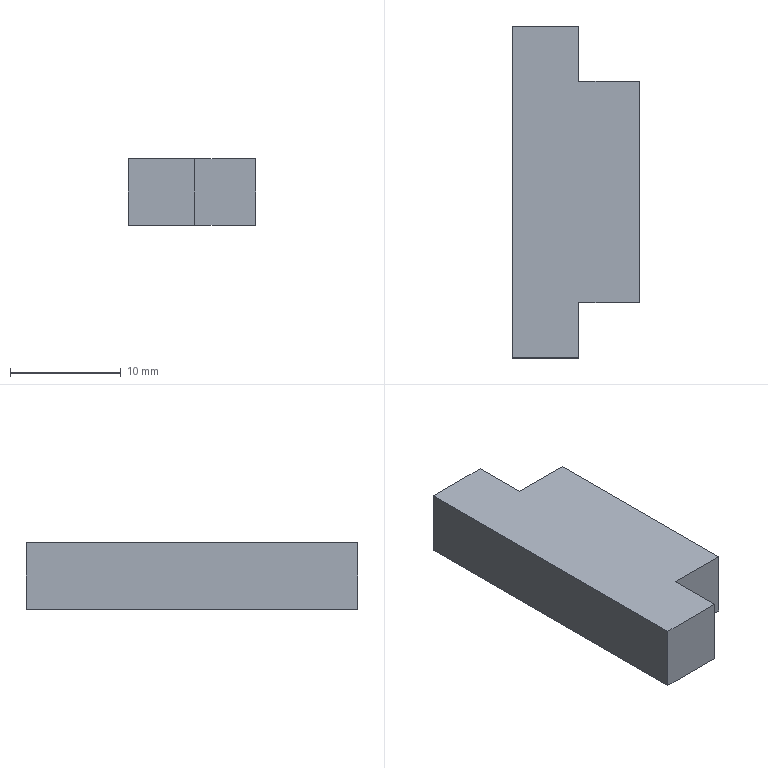Part | SolidWorks | features FlatPattern 1, SMBaseFlange 1, SheetMetal 1 | 1 solid | 10 faces | box 11.5 x 30 x 6 mm | volume 1740 mm3 | plane 10
STEP:
#1=CARTESIAN_POINT('',(11.5,-104.,0.));
#2=VERTEX_POINT('',#1);
#3=CARTESIAN_POINT('',(11.5,-84.,0.));
#4=VERTEX_POINT('',#3);
#5=CARTESIAN_POINT('',(11.5,-84.,0.));
#6=DIRECTION('',(0.,1.,0.));
#7=VECTOR('',#6,1000.);
#8=LINE('',#5,#7);
#9=EDGE_CURVE('',#2,#4,#8,.T.);
#10=ORIENTED_EDGE('',*,*,#9,.T.);
#11=CARTESIAN_POINT('',(11.5,-84.,6.));
#12=VERTEX_POINT('',#11);
#13=CARTESIAN_POINT('',(11.5,-84.,6.));
#14=DIRECTION('',(0.,0.,-1.));
#15=VECTOR('',#14,1000.);
#16=LINE('',#13,#15);
#17=EDGE_CURVE('',#12,#4,#16,.T.);
#18=ORIENTED_EDGE('',*,*,#17,.F.);
#19=CARTESIAN_POINT('',(11.5,-104.,6.));
#20=VERTEX_POINT('',#19);
#21=CARTESIAN_POINT('',(11.5,-84.,6.));
#22=DIRECTION('',(0.,1.,0.));
#23=VECTOR('',#22,1000.);
#24=LINE('',#21,#23);
#25=EDGE_CURVE('',#20,#12,#24,.T.);
#26=ORIENTED_EDGE('',*,*,#25,.F.);
#27=CARTESIAN_POINT('',(11.5,-104.,6.));
#28=DIRECTION('',(0.,0.,-1.));
#29=VECTOR('',#28,1000.);
#30=LINE('',#27,#29);
#31=EDGE_CURVE('',#20,#2,#30,.T.);
#32=ORIENTED_EDGE('',*,*,#31,.T.);
#33=EDGE_LOOP('',(#10,#18,#26,#32));
#34=FACE_OUTER_BOUND('',#33,.T.);
#35=CARTESIAN_POINT('',(11.5,-84.,6.));
#36=DIRECTION('',(-1.,0.,0.));
#37=DIRECTION('',(0.,-1.,0.));
#38=AXIS2_PLACEMENT_3D('',#35,#36,#37);
#39=PLANE('',#38);
#40=ADVANCED_FACE('',(#34),#39,.F.);
#41=CARTESIAN_POINT('',(6.,-84.,0.));
#42=VERTEX_POINT('',#41);
#43=CARTESIAN_POINT('',(6.,-84.,0.));
#44=DIRECTION('',(-1.,0.,0.));
#45=VECTOR('',#44,1000.);
#46=LINE('',#43,#45);
#47=EDGE_CURVE('',#4,#42,#46,.T.);
#48=ORIENTED_EDGE('',*,*,#47,.T.);
#49=CARTESIAN_POINT('',(6.,-84.,6.));
#50=VERTEX_POINT('',#49);
#51=CARTESIAN_POINT('',(6.,-84.,6.));
#52=DIRECTION('',(0.,0.,-1.));
#53=VECTOR('',#52,1000.);
#54=LINE('',#51,#53);
#55=EDGE_CURVE('',#50,#42,#54,.T.);
#56=ORIENTED_EDGE('',*,*,#55,.F.);
#57=CARTESIAN_POINT('',(6.,-84.,6.));
#58=DIRECTION('',(-1.,0.,0.));
#59=VECTOR('',#58,1000.);
#60=LINE('',#57,#59);
#61=EDGE_CURVE('',#12,#50,#60,.T.);
#62=ORIENTED_EDGE('',*,*,#61,.F.);
#63=ORIENTED_EDGE('',*,*,#17,.T.);
#64=EDGE_LOOP('',(#48,#56,#62,#63));
#65=FACE_OUTER_BOUND('',#64,.T.);
#66=CARTESIAN_POINT('',(6.,-84.,6.));
#67=DIRECTION('',(0.,-1.,0.));
#68=DIRECTION('',(0.,0.,-1.));
#69=AXIS2_PLACEMENT_3D('',#66,#67,#68);
#70=PLANE('',#69);
#71=ADVANCED_FACE('',(#65),#70,.F.);
#72=CARTESIAN_POINT('',(6.,-79.,0.));
#73=VERTEX_POINT('',#72);
#74=CARTESIAN_POINT('',(6.,-79.,0.));
#75=DIRECTION('',(0.,1.,0.));
#76=VECTOR('',#75,1000.);
#77=LINE('',#74,#76);
#78=EDGE_CURVE('',#42,#73,#77,.T.);
#79=ORIENTED_EDGE('',*,*,#78,.T.);
#80=CARTESIAN_POINT('',(6.,-79.,6.));
#81=VERTEX_POINT('',#80);
#82=CARTESIAN_POINT('',(6.,-79.,6.));
#83=DIRECTION('',(0.,0.,-1.));
#84=VECTOR('',#83,1000.);
#85=LINE('',#82,#84);
#86=EDGE_CURVE('',#81,#73,#85,.T.);
#87=ORIENTED_EDGE('',*,*,#86,.F.);
#88=CARTESIAN_POINT('',(6.,-79.,6.));
#89=DIRECTION('',(0.,1.,0.));
#90=VECTOR('',#89,1000.);
#91=LINE('',#88,#90);
#92=EDGE_CURVE('',#50,#81,#91,.T.);
#93=ORIENTED_EDGE('',*,*,#92,.F.);
#94=ORIENTED_EDGE('',*,*,#55,.T.);
#95=EDGE_LOOP('',(#79,#87,#93,#94));
#96=FACE_OUTER_BOUND('',#95,.T.);
#97=CARTESIAN_POINT('',(6.,-79.,6.));
#98=DIRECTION('',(-1.,0.,0.));
#99=DIRECTION('',(0.,-1.,0.));
#100=AXIS2_PLACEMENT_3D('',#97,#98,#99);
#101=PLANE('',#100);
#102=ADVANCED_FACE('',(#96),#101,.F.);
#103=CARTESIAN_POINT('',(0.,-79.,0.));
#104=VERTEX_POINT('',#103);
#105=CARTESIAN_POINT('',(0.,-79.,0.));
#106=DIRECTION('',(-1.,0.,0.));
#107=VECTOR('',#106,1000.);
#108=LINE('',#105,#107);
#109=EDGE_CURVE('',#73,#104,#108,.T.);
#110=ORIENTED_EDGE('',*,*,#109,.T.);
#111=CARTESIAN_POINT('',(0.,-79.,6.));
#112=VERTEX_POINT('',#111);
#113=CARTESIAN_POINT('',(0.,-79.,6.));
#114=DIRECTION('',(0.,0.,-1.));
#115=VECTOR('',#114,1000.);
#116=LINE('',#113,#115);
#117=EDGE_CURVE('',#112,#104,#116,.T.);
#118=ORIENTED_EDGE('',*,*,#117,.F.);
#119=CARTESIAN_POINT('',(0.,-79.,6.));
#120=DIRECTION('',(-1.,0.,0.));
#121=VECTOR('',#120,1000.);
#122=LINE('',#119,#121);
#123=EDGE_CURVE('',#81,#112,#122,.T.);
#124=ORIENTED_EDGE('',*,*,#123,.F.);
#125=ORIENTED_EDGE('',*,*,#86,.T.);
#126=EDGE_LOOP('',(#110,#118,#124,#125));
#127=FACE_OUTER_BOUND('',#126,.T.);
#128=CARTESIAN_POINT('',(0.,-79.,6.));
#129=DIRECTION('',(0.,-1.,0.));
#130=DIRECTION('',(0.,0.,-1.));
#131=AXIS2_PLACEMENT_3D('',#128,#129,#130);
#132=PLANE('',#131);
#133=ADVANCED_FACE('',(#127),#132,.F.);
#134=CARTESIAN_POINT('',(0.,-109.,0.));
#135=VERTEX_POINT('',#134);
#136=CARTESIAN_POINT('',(0.,-109.,0.));
#137=DIRECTION('',(0.,-1.,0.));
#138=VECTOR('',#137,1000.);
#139=LINE('',#136,#138);
#140=EDGE_CURVE('',#104,#135,#139,.T.);
#141=ORIENTED_EDGE('',*,*,#140,.T.);
#142=CARTESIAN_POINT('',(0.,-109.,6.));
#143=VERTEX_POINT('',#142);
#144=CARTESIAN_POINT('',(0.,-109.,6.));
#145=DIRECTION('',(0.,0.,-1.));
#146=VECTOR('',#145,1000.);
#147=LINE('',#144,#146);
#148=EDGE_CURVE('',#143,#135,#147,.T.);
#149=ORIENTED_EDGE('',*,*,#148,.F.);
#150=CARTESIAN_POINT('',(0.,-109.,6.));
#151=DIRECTION('',(0.,-1.,0.));
#152=VECTOR('',#151,1000.);
#153=LINE('',#150,#152);
#154=EDGE_CURVE('',#112,#143,#153,.T.);
#155=ORIENTED_EDGE('',*,*,#154,.F.);
#156=ORIENTED_EDGE('',*,*,#117,.T.);
#157=EDGE_LOOP('',(#141,#149,#155,#156));
#158=FACE_OUTER_BOUND('',#157,.T.);
#159=CARTESIAN_POINT('',(0.,-109.,6.));
#160=DIRECTION('',(1.,0.,0.));
#161=DIRECTION('',(0.,0.,-1.));
#162=AXIS2_PLACEMENT_3D('',#159,#160,#161);
#163=PLANE('',#162);
#164=ADVANCED_FACE('',(#158),#163,.F.);
#165=CARTESIAN_POINT('',(6.,-109.,0.));
#166=VERTEX_POINT('',#165);
#167=CARTESIAN_POINT('',(6.,-109.,0.));
#168=DIRECTION('',(1.,0.,0.));
#169=VECTOR('',#168,1000.);
#170=LINE('',#167,#169);
#171=EDGE_CURVE('',#135,#166,#170,.T.);
#172=ORIENTED_EDGE('',*,*,#171,.T.);
#173=CARTESIAN_POINT('',(6.,-109.,6.));
#174=VERTEX_POINT('',#173);
#175=CARTESIAN_POINT('',(6.,-109.,6.));
#176=DIRECTION('',(0.,0.,-1.));
#177=VECTOR('',#176,1000.);
#178=LINE('',#175,#177);
#179=EDGE_CURVE('',#174,#166,#178,.T.);
#180=ORIENTED_EDGE('',*,*,#179,.F.);
#181=CARTESIAN_POINT('',(6.,-109.,6.));
#182=DIRECTION('',(1.,0.,0.));
#183=VECTOR('',#182,1000.);
#184=LINE('',#181,#183);
#185=EDGE_CURVE('',#143,#174,#184,.T.);
#186=ORIENTED_EDGE('',*,*,#185,.F.);
#187=ORIENTED_EDGE('',*,*,#148,.T.);
#188=EDGE_LOOP('',(#172,#180,#186,#187));
#189=FACE_OUTER_BOUND('',#188,.T.);
#190=CARTESIAN_POINT('',(6.,-109.,6.));
#191=DIRECTION('',(0.,1.,0.));
#192=DIRECTION('',(0.,0.,1.));
#193=AXIS2_PLACEMENT_3D('',#190,#191,#192);
#194=PLANE('',#193);
#195=ADVANCED_FACE('',(#189),#194,.F.);
#196=CARTESIAN_POINT('',(6.,-104.,0.));
#197=VERTEX_POINT('',#196);
#198=CARTESIAN_POINT('',(6.,-104.,0.));
#199=DIRECTION('',(0.,1.,0.));
#200=VECTOR('',#199,1000.);
#201=LINE('',#198,#200);
#202=EDGE_CURVE('',#166,#197,#201,.T.);
#203=ORIENTED_EDGE('',*,*,#202,.T.);
#204=CARTESIAN_POINT('',(6.,-104.,6.));
#205=VERTEX_POINT('',#204);
#206=CARTESIAN_POINT('',(6.,-104.,6.));
#207=DIRECTION('',(0.,0.,-1.));
#208=VECTOR('',#207,1000.);
#209=LINE('',#206,#208);
#210=EDGE_CURVE('',#205,#197,#209,.T.);
#211=ORIENTED_EDGE('',*,*,#210,.F.);
#212=CARTESIAN_POINT('',(6.,-104.,6.));
#213=DIRECTION('',(0.,1.,0.));
#214=VECTOR('',#213,1000.);
#215=LINE('',#212,#214);
#216=EDGE_CURVE('',#174,#205,#215,.T.);
#217=ORIENTED_EDGE('',*,*,#216,.F.);
#218=ORIENTED_EDGE('',*,*,#179,.T.);
#219=EDGE_LOOP('',(#203,#211,#217,#218));
#220=FACE_OUTER_BOUND('',#219,.T.);
#221=CARTESIAN_POINT('',(6.,-104.,6.));
#222=DIRECTION('',(-1.,0.,0.));
#223=DIRECTION('',(0.,-1.,0.));
#224=AXIS2_PLACEMENT_3D('',#221,#222,#223);
#225=PLANE('',#224);
#226=ADVANCED_FACE('',(#220),#225,.F.);
#227=CARTESIAN_POINT('',(11.5,-104.,0.));
#228=DIRECTION('',(1.,0.,0.));
#229=VECTOR('',#228,1000.);
#230=LINE('',#227,#229);
#231=EDGE_CURVE('',#197,#2,#230,.T.);
#232=ORIENTED_EDGE('',*,*,#231,.T.);
#233=ORIENTED_EDGE('',*,*,#31,.F.);
#234=CARTESIAN_POINT('',(11.5,-104.,6.));
#235=DIRECTION('',(1.,0.,0.));
#236=VECTOR('',#235,1000.);
#237=LINE('',#234,#236);
#238=EDGE_CURVE('',#205,#20,#237,.T.);
#239=ORIENTED_EDGE('',*,*,#238,.F.);
#240=ORIENTED_EDGE('',*,*,#210,.T.);
#241=EDGE_LOOP('',(#232,#233,#239,#240));
#242=FACE_OUTER_BOUND('',#241,.T.);
#243=CARTESIAN_POINT('',(11.5,-104.,6.));
#244=DIRECTION('',(0.,1.,0.));
#245=DIRECTION('',(0.,0.,1.));
#246=AXIS2_PLACEMENT_3D('',#243,#244,#245);
#247=PLANE('',#246);
#248=ADVANCED_FACE('',(#242),#247,.F.);
#249=ORIENTED_EDGE('',*,*,#25,.T.);
#250=ORIENTED_EDGE('',*,*,#61,.T.);
#251=ORIENTED_EDGE('',*,*,#92,.T.);
#252=ORIENTED_EDGE('',*,*,#123,.T.);
#253=ORIENTED_EDGE('',*,*,#154,.T.);
#254=ORIENTED_EDGE('',*,*,#185,.T.);
#255=ORIENTED_EDGE('',*,*,#216,.T.);
#256=ORIENTED_EDGE('',*,*,#238,.T.);
#257=EDGE_LOOP('',(#249,#250,#251,#252,#253,#254,#255,#256));
#258=FACE_OUTER_BOUND('',#257,.T.);
#259=CARTESIAN_POINT('',(0.,0.,6.));
#260=DIRECTION('',(0.,0.,-1.));
#261=DIRECTION('',(-1.,0.,0.));
#262=AXIS2_PLACEMENT_3D('',#259,#260,#261);
#263=PLANE('',#262);
#264=ADVANCED_FACE('',(#258),#263,.F.);
#265=ORIENTED_EDGE('',*,*,#9,.F.);
#266=ORIENTED_EDGE('',*,*,#231,.F.);
#267=ORIENTED_EDGE('',*,*,#202,.F.);
#268=ORIENTED_EDGE('',*,*,#171,.F.);
#269=ORIENTED_EDGE('',*,*,#140,.F.);
#270=ORIENTED_EDGE('',*,*,#109,.F.);
#271=ORIENTED_EDGE('',*,*,#78,.F.);
#272=ORIENTED_EDGE('',*,*,#47,.F.);
#273=EDGE_LOOP('',(#265,#266,#267,#268,#269,#270,#271,#272));
#274=FACE_OUTER_BOUND('',#273,.T.);
#275=CARTESIAN_POINT('',(0.,0.,0.));
#276=DIRECTION('',(0.,0.,-1.));
#277=DIRECTION('',(-1.,0.,0.));
#278=AXIS2_PLACEMENT_3D('',#275,#276,#277);
#279=PLANE('',#278);
#280=ADVANCED_FACE('',(#274),#279,.T.);
#281=CLOSED_SHELL('',(#40,#71,#102,#133,#164,#195,#226,#248,#264,#280));
#282=MANIFOLD_SOLID_BREP('',#281);
#283=CARTESIAN_POINT('',(0.,0.,0.));
#284=DIRECTION('',(0.,0.,1.));
#285=DIRECTION('',(1.,0.,0.));
#286=AXIS2_PLACEMENT_3D('',#283,#284,#285);
#287=(LENGTH_UNIT()NAMED_UNIT(*)SI_UNIT(.MILLI.,.METRE.));
#288=UNCERTAINTY_MEASURE_WITH_UNIT(LENGTH_MEASURE(0.00001),#287,'','');
#289=(NAMED_UNIT(*)PLANE_ANGLE_UNIT()SI_UNIT($,.RADIAN.));
#290=(NAMED_UNIT(*)SI_UNIT($,.STERADIAN.)SOLID_ANGLE_UNIT());
#291=(GEOMETRIC_REPRESENTATION_CONTEXT(3)GLOBAL_UNCERTAINTY_ASSIGNED_CONTEXT((#288))GLOBAL_UNIT_ASSIGNED_CONTEXT((#287,#289,#290))REPRESENTATION_CONTEXT('',''));
#292=ADVANCED_BREP_SHAPE_REPRESENTATION('',(#282,#286),#291);